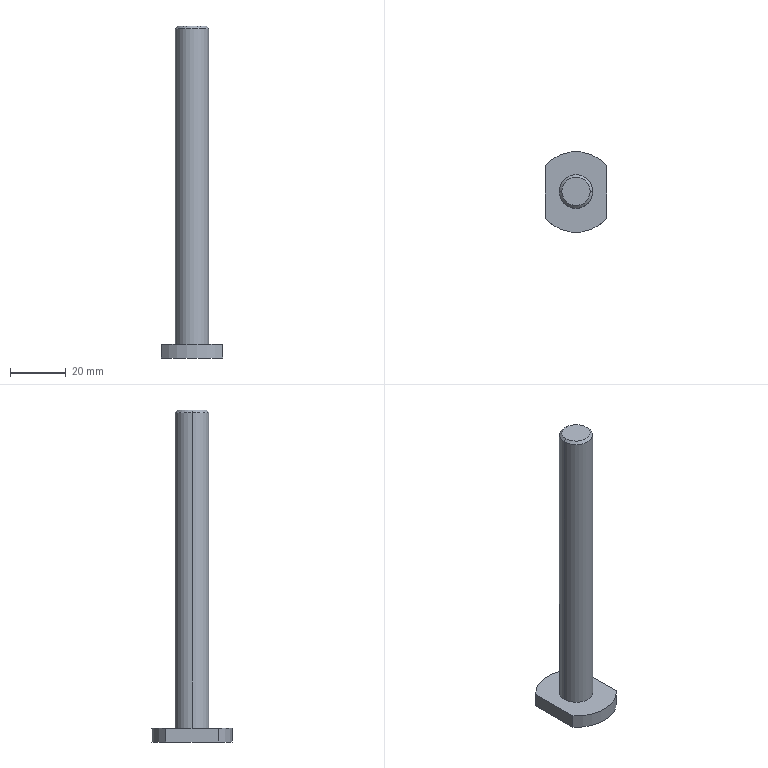Part | SolidWorks | features Chamfer 1, Extrusion 1, ICE 1 | 1 solid | 11 faces | box 22 x 29 x 119.3 mm | volume 15762 mm3 | plane 5 | cylinder 4 | cone 2 | commonest cylinder face diameters 12 x2 29 x2
STEP:
#1=CARTESIAN_POINT('',(5.1,0.,114.3));
#2=VERTEX_POINT('',#1);
#3=CARTESIAN_POINT('',(-5.1,0.,114.3));
#4=VERTEX_POINT('',#3);
#5=CARTESIAN_POINT('',(0.,0.,114.3));
#6=DIRECTION('',(0.,0.,1.));
#7=DIRECTION('',(1.,0.,0.));
#8=AXIS2_PLACEMENT_3D('',#5,#6,#7);
#9=CIRCLE('',#8,5.1);
#10=EDGE_CURVE('',#2,#4,#9,.T.);
#11=ORIENTED_EDGE('',*,*,#10,.F.);
#12=CARTESIAN_POINT('',(6.,0.,113.4));
#13=VERTEX_POINT('',#12);
#14=CARTESIAN_POINT('',(5.1,0.,114.3));
#15=DIRECTION('',(0.7071,0.,-0.7071));
#16=VECTOR('',#15,1000.);
#17=LINE('',#14,#16);
#18=EDGE_CURVE('',#2,#13,#17,.T.);
#19=ORIENTED_EDGE('',*,*,#18,.T.);
#20=CARTESIAN_POINT('',(-6.,0.,113.4));
#21=VERTEX_POINT('',#20);
#22=CARTESIAN_POINT('',(0.,0.,113.4));
#23=DIRECTION('',(0.,0.,-1.));
#24=DIRECTION('',(1.,0.,0.));
#25=AXIS2_PLACEMENT_3D('',#22,#23,#24);
#26=CIRCLE('',#25,6.);
#27=EDGE_CURVE('',#21,#13,#26,.T.);
#28=ORIENTED_EDGE('',*,*,#27,.F.);
#29=CARTESIAN_POINT('',(-5.1,0.,114.3));
#30=DIRECTION('',(-0.7071,0.,-0.7071));
#31=VECTOR('',#30,1000.);
#32=LINE('',#29,#31);
#33=EDGE_CURVE('',#4,#21,#32,.T.);
#34=ORIENTED_EDGE('',*,*,#33,.F.);
#35=EDGE_LOOP('',(#11,#19,#28,#34));
#36=FACE_OUTER_BOUND('',#35,.T.);
#37=CARTESIAN_POINT('',(0.,0.,114.3));
#38=DIRECTION('',(0.,0.,-1.));
#39=DIRECTION('',(-1.,0.,0.));
#40=AXIS2_PLACEMENT_3D('',#37,#38,#39);
#41=CONICAL_SURFACE('',#40,5.1,0.7854);
#42=ADVANCED_FACE('',(#36),#41,.T.);
#43=ORIENTED_EDGE('',*,*,#27,.T.);
#44=CARTESIAN_POINT('',(6.,0.,0.));
#45=VERTEX_POINT('',#44);
#46=CARTESIAN_POINT('',(6.,0.,114.3));
#47=DIRECTION('',(0.,0.,-1.));
#48=VECTOR('',#47,1000.);
#49=LINE('',#46,#48);
#50=EDGE_CURVE('',#13,#45,#49,.T.);
#51=ORIENTED_EDGE('',*,*,#50,.T.);
#52=CARTESIAN_POINT('',(-6.,0.,0.));
#53=VERTEX_POINT('',#52);
#54=CARTESIAN_POINT('',(0.,0.,0.));
#55=DIRECTION('',(0.,0.,-1.));
#56=DIRECTION('',(-1.,0.,0.));
#57=AXIS2_PLACEMENT_3D('',#54,#55,#56);
#58=CIRCLE('',#57,6.);
#59=EDGE_CURVE('',#53,#45,#58,.T.);
#60=ORIENTED_EDGE('',*,*,#59,.F.);
#61=CARTESIAN_POINT('',(-6.,0.,114.3));
#62=DIRECTION('',(0.,0.,-1.));
#63=VECTOR('',#62,1000.);
#64=LINE('',#61,#63);
#65=EDGE_CURVE('',#21,#53,#64,.T.);
#66=ORIENTED_EDGE('',*,*,#65,.F.);
#67=EDGE_LOOP('',(#43,#51,#60,#66));
#68=FACE_OUTER_BOUND('',#67,.T.);
#69=CARTESIAN_POINT('',(0.,0.,114.3));
#70=DIRECTION('',(0.,0.,-1.));
#71=DIRECTION('',(-1.,0.,0.));
#72=AXIS2_PLACEMENT_3D('',#69,#70,#71);
#73=CYLINDRICAL_SURFACE('',#72,6.);
#74=ADVANCED_FACE('',(#68),#73,.T.);
#75=ORIENTED_EDGE('',*,*,#50,.F.);
#76=CARTESIAN_POINT('',(0.,0.,113.4));
#77=DIRECTION('',(0.,0.,-1.));
#78=DIRECTION('',(1.,0.,0.));
#79=AXIS2_PLACEMENT_3D('',#76,#77,#78);
#80=CIRCLE('',#79,6.);
#81=EDGE_CURVE('',#13,#21,#80,.T.);
#82=ORIENTED_EDGE('',*,*,#81,.T.);
#83=ORIENTED_EDGE('',*,*,#65,.T.);
#84=CARTESIAN_POINT('',(0.,0.,0.));
#85=DIRECTION('',(0.,0.,-1.));
#86=DIRECTION('',(-1.,0.,0.));
#87=AXIS2_PLACEMENT_3D('',#84,#85,#86);
#88=CIRCLE('',#87,6.);
#89=EDGE_CURVE('',#45,#53,#88,.T.);
#90=ORIENTED_EDGE('',*,*,#89,.F.);
#91=EDGE_LOOP('',(#75,#82,#83,#90));
#92=FACE_OUTER_BOUND('',#91,.T.);
#93=CARTESIAN_POINT('',(0.,0.,114.3));
#94=DIRECTION('',(0.,0.,-1.));
#95=DIRECTION('',(-1.,0.,0.));
#96=AXIS2_PLACEMENT_3D('',#93,#94,#95);
#97=CYLINDRICAL_SURFACE('',#96,6.);
#98=ADVANCED_FACE('',(#92),#97,.T.);
#99=CARTESIAN_POINT('',(0.,0.,114.3));
#100=DIRECTION('',(0.,0.,1.));
#101=DIRECTION('',(1.,0.,0.));
#102=AXIS2_PLACEMENT_3D('',#99,#100,#101);
#103=CIRCLE('',#102,5.1);
#104=EDGE_CURVE('',#4,#2,#103,.T.);
#105=ORIENTED_EDGE('',*,*,#104,.T.);
#106=ORIENTED_EDGE('',*,*,#10,.T.);
#107=EDGE_LOOP('',(#105,#106));
#108=FACE_OUTER_BOUND('',#107,.T.);
#109=CARTESIAN_POINT('',(0.,0.,114.3));
#110=DIRECTION('',(0.,0.,1.));
#111=DIRECTION('',(1.,0.,0.));
#112=AXIS2_PLACEMENT_3D('',#109,#110,#111);
#113=PLANE('',#112);
#114=ADVANCED_FACE('',(#108),#113,.T.);
#115=ORIENTED_EDGE('',*,*,#18,.F.);
#116=ORIENTED_EDGE('',*,*,#104,.F.);
#117=ORIENTED_EDGE('',*,*,#33,.T.);
#118=ORIENTED_EDGE('',*,*,#81,.F.);
#119=EDGE_LOOP('',(#115,#116,#117,#118));
#120=FACE_OUTER_BOUND('',#119,.T.);
#121=CARTESIAN_POINT('',(0.,0.,114.3));
#122=DIRECTION('',(0.,0.,-1.));
#123=DIRECTION('',(-1.,0.,0.));
#124=AXIS2_PLACEMENT_3D('',#121,#122,#123);
#125=CONICAL_SURFACE('',#124,5.1,0.7854);
#126=ADVANCED_FACE('',(#120),#125,.T.);
#127=CARTESIAN_POINT('',(-11.,9.447,0.));
#128=VERTEX_POINT('',#127);
#129=CARTESIAN_POINT('',(-11.,-9.447,0.));
#130=VERTEX_POINT('',#129);
#131=CARTESIAN_POINT('',(-11.,9.447,0.));
#132=DIRECTION('',(0.,-1.,0.));
#133=VECTOR('',#132,1000.);
#134=LINE('',#131,#133);
#135=EDGE_CURVE('',#128,#130,#134,.T.);
#136=ORIENTED_EDGE('',*,*,#135,.T.);
#137=CARTESIAN_POINT('',(11.,-9.447,0.));
#138=VERTEX_POINT('',#137);
#139=CARTESIAN_POINT('',(0.,0.,0.));
#140=DIRECTION('',(0.,0.,-1.));
#141=DIRECTION('',(-1.,0.,0.));
#142=AXIS2_PLACEMENT_3D('',#139,#140,#141);
#143=CIRCLE('',#142,14.5);
#144=EDGE_CURVE('',#138,#130,#143,.T.);
#145=ORIENTED_EDGE('',*,*,#144,.F.);
#146=CARTESIAN_POINT('',(11.,9.447,0.));
#147=VERTEX_POINT('',#146);
#148=CARTESIAN_POINT('',(11.,9.447,0.));
#149=DIRECTION('',(0.,-1.,0.));
#150=VECTOR('',#149,1000.);
#151=LINE('',#148,#150);
#152=EDGE_CURVE('',#147,#138,#151,.T.);
#153=ORIENTED_EDGE('',*,*,#152,.F.);
#154=CARTESIAN_POINT('',(0.,0.,0.));
#155=DIRECTION('',(0.,0.,-1.));
#156=DIRECTION('',(-1.,0.,0.));
#157=AXIS2_PLACEMENT_3D('',#154,#155,#156);
#158=CIRCLE('',#157,14.5);
#159=EDGE_CURVE('',#128,#147,#158,.T.);
#160=ORIENTED_EDGE('',*,*,#159,.F.);
#161=EDGE_LOOP('',(#136,#145,#153,#160));
#162=FACE_OUTER_BOUND('',#161,.T.);
#163=ORIENTED_EDGE('',*,*,#59,.T.);
#164=ORIENTED_EDGE('',*,*,#89,.T.);
#165=EDGE_LOOP('',(#163,#164));
#166=FACE_BOUND('',#165,.T.);
#167=CARTESIAN_POINT('',(0.,0.,0.));
#168=DIRECTION('',(0.,0.,-1.));
#169=DIRECTION('',(-1.,0.,0.));
#170=AXIS2_PLACEMENT_3D('',#167,#168,#169);
#171=PLANE('',#170);
#172=ADVANCED_FACE('',(#162,#166),#171,.F.);
#173=ORIENTED_EDGE('',*,*,#135,.F.);
#174=CARTESIAN_POINT('',(-11.,9.447,-5.));
#175=VERTEX_POINT('',#174);
#176=CARTESIAN_POINT('',(-11.,9.447,-5.));
#177=DIRECTION('',(0.,0.,1.));
#178=VECTOR('',#177,1000.);
#179=LINE('',#176,#178);
#180=EDGE_CURVE('',#175,#128,#179,.T.);
#181=ORIENTED_EDGE('',*,*,#180,.F.);
#182=CARTESIAN_POINT('',(-11.,-9.447,-5.));
#183=VERTEX_POINT('',#182);
#184=CARTESIAN_POINT('',(-11.,9.447,-5.));
#185=DIRECTION('',(0.,-1.,0.));
#186=VECTOR('',#185,1000.);
#187=LINE('',#184,#186);
#188=EDGE_CURVE('',#175,#183,#187,.T.);
#189=ORIENTED_EDGE('',*,*,#188,.T.);
#190=CARTESIAN_POINT('',(-11.,-9.447,-5.));
#191=DIRECTION('',(0.,0.,1.));
#192=VECTOR('',#191,1000.);
#193=LINE('',#190,#192);
#194=EDGE_CURVE('',#183,#130,#193,.T.);
#195=ORIENTED_EDGE('',*,*,#194,.T.);
#196=EDGE_LOOP('',(#173,#181,#189,#195));
#197=FACE_OUTER_BOUND('',#196,.T.);
#198=CARTESIAN_POINT('',(-11.,9.447,-5.));
#199=DIRECTION('',(-1.,0.,0.));
#200=DIRECTION('',(0.,0.,1.));
#201=AXIS2_PLACEMENT_3D('',#198,#199,#200);
#202=PLANE('',#201);
#203=ADVANCED_FACE('',(#197),#202,.T.);
#204=ORIENTED_EDGE('',*,*,#159,.T.);
#205=CARTESIAN_POINT('',(11.,9.447,-5.));
#206=VERTEX_POINT('',#205);
#207=CARTESIAN_POINT('',(11.,9.447,-5.));
#208=DIRECTION('',(0.,0.,1.));
#209=VECTOR('',#208,1000.);
#210=LINE('',#207,#209);
#211=EDGE_CURVE('',#206,#147,#210,.T.);
#212=ORIENTED_EDGE('',*,*,#211,.F.);
#213=CARTESIAN_POINT('',(0.,0.,-5.));
#214=DIRECTION('',(0.,0.,-1.));
#215=DIRECTION('',(-1.,0.,0.));
#216=AXIS2_PLACEMENT_3D('',#213,#214,#215);
#217=CIRCLE('',#216,14.5);
#218=EDGE_CURVE('',#175,#206,#217,.T.);
#219=ORIENTED_EDGE('',*,*,#218,.F.);
#220=ORIENTED_EDGE('',*,*,#180,.T.);
#221=EDGE_LOOP('',(#204,#212,#219,#220));
#222=FACE_OUTER_BOUND('',#221,.T.);
#223=CARTESIAN_POINT('',(0.,0.,-5.));
#224=DIRECTION('',(0.,0.,1.));
#225=DIRECTION('',(1.,0.,0.));
#226=AXIS2_PLACEMENT_3D('',#223,#224,#225);
#227=CYLINDRICAL_SURFACE('',#226,14.5);
#228=ADVANCED_FACE('',(#222),#227,.T.);
#229=ORIENTED_EDGE('',*,*,#152,.T.);
#230=CARTESIAN_POINT('',(11.,-9.447,-5.));
#231=VERTEX_POINT('',#230);
#232=CARTESIAN_POINT('',(11.,-9.447,-5.));
#233=DIRECTION('',(0.,0.,1.));
#234=VECTOR('',#233,1000.);
#235=LINE('',#232,#234);
#236=EDGE_CURVE('',#231,#138,#235,.T.);
#237=ORIENTED_EDGE('',*,*,#236,.F.);
#238=CARTESIAN_POINT('',(11.,9.447,-5.));
#239=DIRECTION('',(0.,-1.,0.));
#240=VECTOR('',#239,1000.);
#241=LINE('',#238,#240);
#242=EDGE_CURVE('',#206,#231,#241,.T.);
#243=ORIENTED_EDGE('',*,*,#242,.F.);
#244=ORIENTED_EDGE('',*,*,#211,.T.);
#245=EDGE_LOOP('',(#229,#237,#243,#244));
#246=FACE_OUTER_BOUND('',#245,.T.);
#247=CARTESIAN_POINT('',(11.,9.447,-5.));
#248=DIRECTION('',(-1.,0.,0.));
#249=DIRECTION('',(0.,-1.,0.));
#250=AXIS2_PLACEMENT_3D('',#247,#248,#249);
#251=PLANE('',#250);
#252=ADVANCED_FACE('',(#246),#251,.F.);
#253=ORIENTED_EDGE('',*,*,#144,.T.);
#254=ORIENTED_EDGE('',*,*,#194,.F.);
#255=CARTESIAN_POINT('',(0.,0.,-5.));
#256=DIRECTION('',(0.,0.,-1.));
#257=DIRECTION('',(-1.,0.,0.));
#258=AXIS2_PLACEMENT_3D('',#255,#256,#257);
#259=CIRCLE('',#258,14.5);
#260=EDGE_CURVE('',#231,#183,#259,.T.);
#261=ORIENTED_EDGE('',*,*,#260,.F.);
#262=ORIENTED_EDGE('',*,*,#236,.T.);
#263=EDGE_LOOP('',(#253,#254,#261,#262));
#264=FACE_OUTER_BOUND('',#263,.T.);
#265=CARTESIAN_POINT('',(0.,0.,-5.));
#266=DIRECTION('',(0.,0.,1.));
#267=DIRECTION('',(1.,0.,0.));
#268=AXIS2_PLACEMENT_3D('',#265,#266,#267);
#269=CYLINDRICAL_SURFACE('',#268,14.5);
#270=ADVANCED_FACE('',(#264),#269,.T.);
#271=ORIENTED_EDGE('',*,*,#188,.F.);
#272=ORIENTED_EDGE('',*,*,#218,.T.);
#273=ORIENTED_EDGE('',*,*,#242,.T.);
#274=ORIENTED_EDGE('',*,*,#260,.T.);
#275=EDGE_LOOP('',(#271,#272,#273,#274));
#276=FACE_OUTER_BOUND('',#275,.T.);
#277=CARTESIAN_POINT('',(0.,0.,-5.));
#278=DIRECTION('',(0.,0.,-1.));
#279=DIRECTION('',(-1.,0.,0.));
#280=AXIS2_PLACEMENT_3D('',#277,#278,#279);
#281=PLANE('',#280);
#282=ADVANCED_FACE('',(#276),#281,.T.);
#283=CLOSED_SHELL('',(#42,#74,#98,#114,#126,#172,#203,#228,#252,#270,#282));
#284=MANIFOLD_SOLID_BREP('',#283);
#285=CARTESIAN_POINT('',(0.,0.,0.));
#286=DIRECTION('',(0.,0.,1.));
#287=DIRECTION('',(1.,0.,0.));
#288=AXIS2_PLACEMENT_3D('',#285,#286,#287);
#289=(LENGTH_UNIT()NAMED_UNIT(*)SI_UNIT(.MILLI.,.METRE.));
#290=UNCERTAINTY_MEASURE_WITH_UNIT(LENGTH_MEASURE(0.00001),#289,'','');
#291=(NAMED_UNIT(*)PLANE_ANGLE_UNIT()SI_UNIT($,.RADIAN.));
#292=(NAMED_UNIT(*)SI_UNIT($,.STERADIAN.)SOLID_ANGLE_UNIT());
#293=(GEOMETRIC_REPRESENTATION_CONTEXT(3)GLOBAL_UNCERTAINTY_ASSIGNED_CONTEXT((#290))GLOBAL_UNIT_ASSIGNED_CONTEXT((#289,#291,#292))REPRESENTATION_CONTEXT('',''));
#294=ADVANCED_BREP_SHAPE_REPRESENTATION('',(#284,#288),#293);